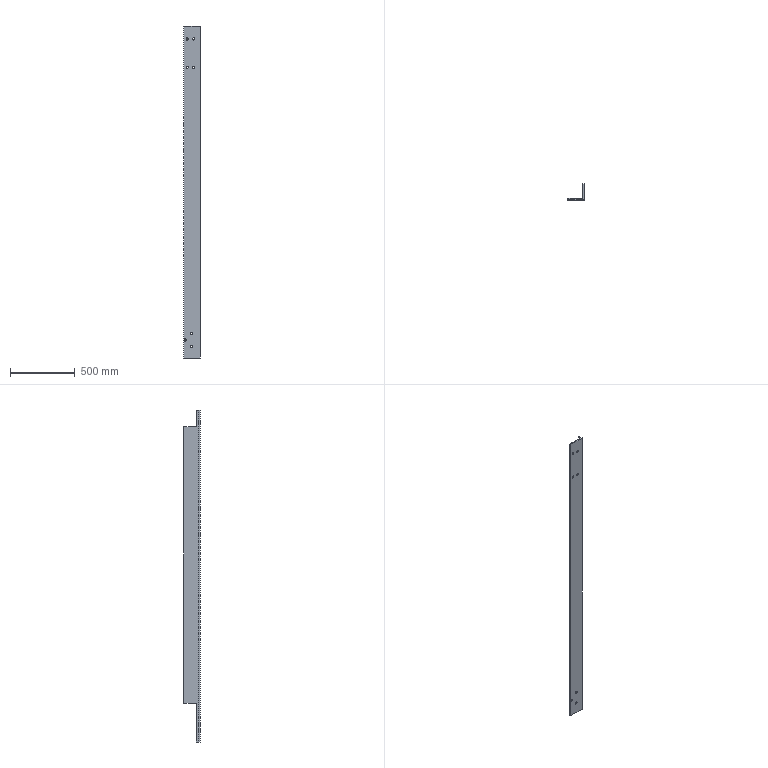Part | SolidWorks | features MirrorStock 1 | 1 solid | 26 faces | box 125 x 125 x 2570 mm | volume 5742663 mm3 | cylinder 14 | plane 12 | commonest cylinder face diameters 17.5 x14
STEP:
#1=CARTESIAN_POINT('',(-100.,0.,956.25));
#2=VERTEX_POINT('',#1);
#3=CARTESIAN_POINT('',(-100.,0.,973.75));
#4=VERTEX_POINT('',#3);
#5=CARTESIAN_POINT('',(-100.,0.,965.));
#6=DIRECTION('',(0.,-1.,0.));
#7=DIRECTION('',(0.,0.,-1.));
#8=AXIS2_PLACEMENT_3D('',#5,#6,#7);
#9=CIRCLE('',#8,8.75);
#10=EDGE_CURVE('',#2,#4,#9,.T.);
#11=ORIENTED_EDGE('',*,*,#10,.T.);
#12=CARTESIAN_POINT('',(-100.,10.,973.75));
#13=VERTEX_POINT('',#12);
#14=CARTESIAN_POINT('',(-100.,10.,973.75));
#15=DIRECTION('',(0.,1.,0.));
#16=VECTOR('',#15,1000.);
#17=LINE('',#14,#16);
#18=EDGE_CURVE('',#4,#13,#17,.T.);
#19=ORIENTED_EDGE('',*,*,#18,.T.);
#20=CARTESIAN_POINT('',(-100.,10.,956.25));
#21=VERTEX_POINT('',#20);
#22=CARTESIAN_POINT('',(-100.,10.,965.));
#23=DIRECTION('',(0.,-1.,0.));
#24=DIRECTION('',(0.,0.,-1.));
#25=AXIS2_PLACEMENT_3D('',#22,#23,#24);
#26=CIRCLE('',#25,8.75);
#27=EDGE_CURVE('',#21,#13,#26,.T.);
#28=ORIENTED_EDGE('',*,*,#27,.F.);
#29=CARTESIAN_POINT('',(-100.,10.,956.25));
#30=DIRECTION('',(0.,1.,0.));
#31=VECTOR('',#30,1000.);
#32=LINE('',#29,#31);
#33=EDGE_CURVE('',#2,#21,#32,.T.);
#34=ORIENTED_EDGE('',*,*,#33,.F.);
#35=EDGE_LOOP('',(#11,#19,#28,#34));
#36=FACE_OUTER_BOUND('',#35,.T.);
#37=CARTESIAN_POINT('',(-100.,10.,965.));
#38=DIRECTION('',(0.,1.,0.));
#39=DIRECTION('',(0.,0.,-1.));
#40=AXIS2_PLACEMENT_3D('',#37,#38,#39);
#41=CYLINDRICAL_SURFACE('',#40,8.75);
#42=ADVANCED_FACE('',(#36),#41,.F.);
#43=CARTESIAN_POINT('',(-50.,0.,956.25));
#44=VERTEX_POINT('',#43);
#45=CARTESIAN_POINT('',(-50.,0.,973.75));
#46=VERTEX_POINT('',#45);
#47=CARTESIAN_POINT('',(-50.,0.,965.));
#48=DIRECTION('',(0.,-1.,0.));
#49=DIRECTION('',(0.,0.,-1.));
#50=AXIS2_PLACEMENT_3D('',#47,#48,#49);
#51=CIRCLE('',#50,8.75);
#52=EDGE_CURVE('',#44,#46,#51,.T.);
#53=ORIENTED_EDGE('',*,*,#52,.T.);
#54=CARTESIAN_POINT('',(-50.,10.,973.75));
#55=VERTEX_POINT('',#54);
#56=CARTESIAN_POINT('',(-50.,10.,973.75));
#57=DIRECTION('',(0.,1.,0.));
#58=VECTOR('',#57,1000.);
#59=LINE('',#56,#58);
#60=EDGE_CURVE('',#46,#55,#59,.T.);
#61=ORIENTED_EDGE('',*,*,#60,.T.);
#62=CARTESIAN_POINT('',(-50.,10.,956.25));
#63=VERTEX_POINT('',#62);
#64=CARTESIAN_POINT('',(-50.,10.,965.));
#65=DIRECTION('',(0.,-1.,0.));
#66=DIRECTION('',(0.,0.,-1.));
#67=AXIS2_PLACEMENT_3D('',#64,#65,#66);
#68=CIRCLE('',#67,8.75);
#69=EDGE_CURVE('',#63,#55,#68,.T.);
#70=ORIENTED_EDGE('',*,*,#69,.F.);
#71=CARTESIAN_POINT('',(-50.,10.,956.25));
#72=DIRECTION('',(0.,1.,0.));
#73=VECTOR('',#72,1000.);
#74=LINE('',#71,#73);
#75=EDGE_CURVE('',#44,#63,#74,.T.);
#76=ORIENTED_EDGE('',*,*,#75,.F.);
#77=EDGE_LOOP('',(#53,#61,#70,#76));
#78=FACE_OUTER_BOUND('',#77,.T.);
#79=CARTESIAN_POINT('',(-50.,10.,965.));
#80=DIRECTION('',(0.,1.,0.));
#81=DIRECTION('',(0.,0.,-1.));
#82=AXIS2_PLACEMENT_3D('',#79,#80,#81);
#83=CYLINDRICAL_SURFACE('',#82,8.75);
#84=ADVANCED_FACE('',(#78),#83,.F.);
#85=CARTESIAN_POINT('',(-50.,0.,1176.25));
#86=VERTEX_POINT('',#85);
#87=CARTESIAN_POINT('',(-50.,0.,1193.75));
#88=VERTEX_POINT('',#87);
#89=CARTESIAN_POINT('',(-50.,0.,1185.));
#90=DIRECTION('',(0.,-1.,0.));
#91=DIRECTION('',(0.,0.,-1.));
#92=AXIS2_PLACEMENT_3D('',#89,#90,#91);
#93=CIRCLE('',#92,8.75);
#94=EDGE_CURVE('',#86,#88,#93,.T.);
#95=ORIENTED_EDGE('',*,*,#94,.T.);
#96=CARTESIAN_POINT('',(-50.,10.,1193.75));
#97=VERTEX_POINT('',#96);
#98=CARTESIAN_POINT('',(-50.,10.,1193.75));
#99=DIRECTION('',(0.,1.,0.));
#100=VECTOR('',#99,1000.);
#101=LINE('',#98,#100);
#102=EDGE_CURVE('',#88,#97,#101,.T.);
#103=ORIENTED_EDGE('',*,*,#102,.T.);
#104=CARTESIAN_POINT('',(-50.,10.,1176.25));
#105=VERTEX_POINT('',#104);
#106=CARTESIAN_POINT('',(-50.,10.,1185.));
#107=DIRECTION('',(0.,-1.,0.));
#108=DIRECTION('',(0.,0.,-1.));
#109=AXIS2_PLACEMENT_3D('',#106,#107,#108);
#110=CIRCLE('',#109,8.75);
#111=EDGE_CURVE('',#105,#97,#110,.T.);
#112=ORIENTED_EDGE('',*,*,#111,.F.);
#113=CARTESIAN_POINT('',(-50.,10.,1176.25));
#114=DIRECTION('',(0.,1.,0.));
#115=VECTOR('',#114,1000.);
#116=LINE('',#113,#115);
#117=EDGE_CURVE('',#86,#105,#116,.T.);
#118=ORIENTED_EDGE('',*,*,#117,.F.);
#119=EDGE_LOOP('',(#95,#103,#112,#118));
#120=FACE_OUTER_BOUND('',#119,.T.);
#121=CARTESIAN_POINT('',(-50.,10.,1185.));
#122=DIRECTION('',(0.,1.,0.));
#123=DIRECTION('',(0.,0.,-1.));
#124=AXIS2_PLACEMENT_3D('',#121,#122,#123);
#125=CYLINDRICAL_SURFACE('',#124,8.75);
#126=ADVANCED_FACE('',(#120),#125,.F.);
#127=CARTESIAN_POINT('',(-100.,0.,1176.25));
#128=VERTEX_POINT('',#127);
#129=CARTESIAN_POINT('',(-100.,0.,1193.75));
#130=VERTEX_POINT('',#129);
#131=CARTESIAN_POINT('',(-100.,0.,1185.));
#132=DIRECTION('',(0.,-1.,0.));
#133=DIRECTION('',(0.,0.,-1.));
#134=AXIS2_PLACEMENT_3D('',#131,#132,#133);
#135=CIRCLE('',#134,8.75);
#136=EDGE_CURVE('',#128,#130,#135,.T.);
#137=ORIENTED_EDGE('',*,*,#136,.T.);
#138=CARTESIAN_POINT('',(-100.,10.,1193.75));
#139=VERTEX_POINT('',#138);
#140=CARTESIAN_POINT('',(-100.,10.,1193.75));
#141=DIRECTION('',(0.,1.,0.));
#142=VECTOR('',#141,1000.);
#143=LINE('',#140,#142);
#144=EDGE_CURVE('',#130,#139,#143,.T.);
#145=ORIENTED_EDGE('',*,*,#144,.T.);
#146=CARTESIAN_POINT('',(-100.,10.,1176.25));
#147=VERTEX_POINT('',#146);
#148=CARTESIAN_POINT('',(-100.,10.,1185.));
#149=DIRECTION('',(0.,-1.,0.));
#150=DIRECTION('',(0.,0.,-1.));
#151=AXIS2_PLACEMENT_3D('',#148,#149,#150);
#152=CIRCLE('',#151,8.75);
#153=EDGE_CURVE('',#147,#139,#152,.T.);
#154=ORIENTED_EDGE('',*,*,#153,.F.);
#155=CARTESIAN_POINT('',(-100.,10.,1176.25));
#156=DIRECTION('',(0.,1.,0.));
#157=VECTOR('',#156,1000.);
#158=LINE('',#155,#157);
#159=EDGE_CURVE('',#128,#147,#158,.T.);
#160=ORIENTED_EDGE('',*,*,#159,.F.);
#161=EDGE_LOOP('',(#137,#145,#154,#160));
#162=FACE_OUTER_BOUND('',#161,.T.);
#163=CARTESIAN_POINT('',(-100.,10.,1185.));
#164=DIRECTION('',(0.,1.,0.));
#165=DIRECTION('',(0.,0.,-1.));
#166=AXIS2_PLACEMENT_3D('',#163,#164,#165);
#167=CYLINDRICAL_SURFACE('',#166,8.75);
#168=ADVANCED_FACE('',(#162),#167,.F.);
#169=CARTESIAN_POINT('',(-115.,0.,-1153.75));
#170=VERTEX_POINT('',#169);
#171=CARTESIAN_POINT('',(-115.,0.,-1136.25));
#172=VERTEX_POINT('',#171);
#173=CARTESIAN_POINT('',(-115.,0.,-1145.));
#174=DIRECTION('',(0.,-1.,0.));
#175=DIRECTION('',(0.,0.,-1.));
#176=AXIS2_PLACEMENT_3D('',#173,#174,#175);
#177=CIRCLE('',#176,8.75);
#178=EDGE_CURVE('',#170,#172,#177,.T.);
#179=ORIENTED_EDGE('',*,*,#178,.T.);
#180=CARTESIAN_POINT('',(-115.,10.,-1136.25));
#181=VERTEX_POINT('',#180);
#182=CARTESIAN_POINT('',(-115.,10.,-1136.25));
#183=DIRECTION('',(0.,1.,0.));
#184=VECTOR('',#183,1000.);
#185=LINE('',#182,#184);
#186=EDGE_CURVE('',#172,#181,#185,.T.);
#187=ORIENTED_EDGE('',*,*,#186,.T.);
#188=CARTESIAN_POINT('',(-115.,10.,-1153.75));
#189=VERTEX_POINT('',#188);
#190=CARTESIAN_POINT('',(-115.,10.,-1145.));
#191=DIRECTION('',(0.,-1.,0.));
#192=DIRECTION('',(0.,0.,-1.));
#193=AXIS2_PLACEMENT_3D('',#190,#191,#192);
#194=CIRCLE('',#193,8.75);
#195=EDGE_CURVE('',#189,#181,#194,.T.);
#196=ORIENTED_EDGE('',*,*,#195,.F.);
#197=CARTESIAN_POINT('',(-115.,10.,-1153.75));
#198=DIRECTION('',(0.,1.,0.));
#199=VECTOR('',#198,1000.);
#200=LINE('',#197,#199);
#201=EDGE_CURVE('',#170,#189,#200,.T.);
#202=ORIENTED_EDGE('',*,*,#201,.F.);
#203=EDGE_LOOP('',(#179,#187,#196,#202));
#204=FACE_OUTER_BOUND('',#203,.T.);
#205=CARTESIAN_POINT('',(-115.,10.,-1145.));
#206=DIRECTION('',(0.,1.,0.));
#207=DIRECTION('',(0.,0.,-1.));
#208=AXIS2_PLACEMENT_3D('',#205,#206,#207);
#209=CYLINDRICAL_SURFACE('',#208,8.75);
#210=ADVANCED_FACE('',(#204),#209,.F.);
#211=CARTESIAN_POINT('',(-65.,0.,-1103.75));
#212=VERTEX_POINT('',#211);
#213=CARTESIAN_POINT('',(-65.,0.,-1086.25));
#214=VERTEX_POINT('',#213);
#215=CARTESIAN_POINT('',(-65.,0.,-1095.));
#216=DIRECTION('',(0.,-1.,0.));
#217=DIRECTION('',(0.,0.,-1.));
#218=AXIS2_PLACEMENT_3D('',#215,#216,#217);
#219=CIRCLE('',#218,8.75);
#220=EDGE_CURVE('',#212,#214,#219,.T.);
#221=ORIENTED_EDGE('',*,*,#220,.T.);
#222=CARTESIAN_POINT('',(-65.,10.,-1086.25));
#223=VERTEX_POINT('',#222);
#224=CARTESIAN_POINT('',(-65.,10.,-1086.25));
#225=DIRECTION('',(0.,1.,0.));
#226=VECTOR('',#225,1000.);
#227=LINE('',#224,#226);
#228=EDGE_CURVE('',#214,#223,#227,.T.);
#229=ORIENTED_EDGE('',*,*,#228,.T.);
#230=CARTESIAN_POINT('',(-65.,10.,-1103.75));
#231=VERTEX_POINT('',#230);
#232=CARTESIAN_POINT('',(-65.,10.,-1095.));
#233=DIRECTION('',(0.,-1.,0.));
#234=DIRECTION('',(0.,0.,-1.));
#235=AXIS2_PLACEMENT_3D('',#232,#233,#234);
#236=CIRCLE('',#235,8.75);
#237=EDGE_CURVE('',#231,#223,#236,.T.);
#238=ORIENTED_EDGE('',*,*,#237,.F.);
#239=CARTESIAN_POINT('',(-65.,10.,-1103.75));
#240=DIRECTION('',(0.,1.,0.));
#241=VECTOR('',#240,1000.);
#242=LINE('',#239,#241);
#243=EDGE_CURVE('',#212,#231,#242,.T.);
#244=ORIENTED_EDGE('',*,*,#243,.F.);
#245=EDGE_LOOP('',(#221,#229,#238,#244));
#246=FACE_OUTER_BOUND('',#245,.T.);
#247=CARTESIAN_POINT('',(-65.,10.,-1095.));
#248=DIRECTION('',(0.,1.,0.));
#249=DIRECTION('',(0.,0.,-1.));
#250=AXIS2_PLACEMENT_3D('',#247,#248,#249);
#251=CYLINDRICAL_SURFACE('',#250,8.75);
#252=ADVANCED_FACE('',(#246),#251,.F.);
#253=CARTESIAN_POINT('',(-65.,0.,-1203.75));
#254=VERTEX_POINT('',#253);
#255=CARTESIAN_POINT('',(-65.,0.,-1186.25));
#256=VERTEX_POINT('',#255);
#257=CARTESIAN_POINT('',(-65.,0.,-1195.));
#258=DIRECTION('',(0.,-1.,0.));
#259=DIRECTION('',(0.,0.,-1.));
#260=AXIS2_PLACEMENT_3D('',#257,#258,#259);
#261=CIRCLE('',#260,8.75);
#262=EDGE_CURVE('',#254,#256,#261,.T.);
#263=ORIENTED_EDGE('',*,*,#262,.T.);
#264=CARTESIAN_POINT('',(-65.,10.,-1186.25));
#265=VERTEX_POINT('',#264);
#266=CARTESIAN_POINT('',(-65.,10.,-1186.25));
#267=DIRECTION('',(0.,1.,0.));
#268=VECTOR('',#267,1000.);
#269=LINE('',#266,#268);
#270=EDGE_CURVE('',#256,#265,#269,.T.);
#271=ORIENTED_EDGE('',*,*,#270,.T.);
#272=CARTESIAN_POINT('',(-65.,10.,-1203.75));
#273=VERTEX_POINT('',#272);
#274=CARTESIAN_POINT('',(-65.,10.,-1195.));
#275=DIRECTION('',(0.,-1.,0.));
#276=DIRECTION('',(0.,0.,-1.));
#277=AXIS2_PLACEMENT_3D('',#274,#275,#276);
#278=CIRCLE('',#277,8.75);
#279=EDGE_CURVE('',#273,#265,#278,.T.);
#280=ORIENTED_EDGE('',*,*,#279,.F.);
#281=CARTESIAN_POINT('',(-65.,10.,-1203.75));
#282=DIRECTION('',(0.,1.,0.));
#283=VECTOR('',#282,1000.);
#284=LINE('',#281,#283);
#285=EDGE_CURVE('',#254,#273,#284,.T.);
#286=ORIENTED_EDGE('',*,*,#285,.F.);
#287=EDGE_LOOP('',(#263,#271,#280,#286));
#288=FACE_OUTER_BOUND('',#287,.T.);
#289=CARTESIAN_POINT('',(-65.,10.,-1195.));
#290=DIRECTION('',(0.,1.,0.));
#291=DIRECTION('',(0.,0.,-1.));
#292=AXIS2_PLACEMENT_3D('',#289,#290,#291);
#293=CYLINDRICAL_SURFACE('',#292,8.75);
#294=ADVANCED_FACE('',(#288),#293,.F.);
#295=CARTESIAN_POINT('',(-125.,10.,1285.));
#296=VERTEX_POINT('',#295);
#297=CARTESIAN_POINT('',(-125.,0.,1285.));
#298=VERTEX_POINT('',#297);
#299=CARTESIAN_POINT('',(-125.,10.,1285.));
#300=DIRECTION('',(0.,-1.,0.));
#301=VECTOR('',#300,1000.);
#302=LINE('',#299,#301);
#303=EDGE_CURVE('',#296,#298,#302,.T.);
#304=ORIENTED_EDGE('',*,*,#303,.F.);
#305=CARTESIAN_POINT('',(-125.,10.,-1285.));
#306=VERTEX_POINT('',#305);
#307=CARTESIAN_POINT('',(-125.,10.,-1285.));
#308=DIRECTION('',(0.,0.,1.));
#309=VECTOR('',#308,1000.);
#310=LINE('',#307,#309);
#311=EDGE_CURVE('',#306,#296,#310,.T.);
#312=ORIENTED_EDGE('',*,*,#311,.F.);
#313=CARTESIAN_POINT('',(-125.,0.,-1285.));
#314=VERTEX_POINT('',#313);
#315=CARTESIAN_POINT('',(-125.,10.,-1285.));
#316=DIRECTION('',(0.,-1.,0.));
#317=VECTOR('',#316,1000.);
#318=LINE('',#315,#317);
#319=EDGE_CURVE('',#306,#314,#318,.T.);
#320=ORIENTED_EDGE('',*,*,#319,.T.);
#321=CARTESIAN_POINT('',(-125.,0.,-1285.));
#322=DIRECTION('',(0.,0.,1.));
#323=VECTOR('',#322,1000.);
#324=LINE('',#321,#323);
#325=EDGE_CURVE('',#314,#298,#324,.T.);
#326=ORIENTED_EDGE('',*,*,#325,.T.);
#327=EDGE_LOOP('',(#304,#312,#320,#326));
#328=FACE_OUTER_BOUND('',#327,.T.);
#329=CARTESIAN_POINT('',(-125.,10.,-1285.));
#330=DIRECTION('',(1.,0.,0.));
#331=DIRECTION('',(0.,0.,1.));
#332=AXIS2_PLACEMENT_3D('',#329,#330,#331);
#333=PLANE('',#332);
#334=ADVANCED_FACE('',(#328),#333,.F.);
#335=ORIENTED_EDGE('',*,*,#10,.F.);
#336=CARTESIAN_POINT('',(-100.,0.,965.));
#337=DIRECTION('',(0.,-1.,0.));
#338=DIRECTION('',(0.,0.,-1.));
#339=AXIS2_PLACEMENT_3D('',#336,#337,#338);
#340=CIRCLE('',#339,8.75);
#341=EDGE_CURVE('',#4,#2,#340,.T.);
#342=ORIENTED_EDGE('',*,*,#341,.F.);
#343=EDGE_LOOP('',(#335,#342));
#344=FACE_BOUND('',#343,.T.);
#345=ORIENTED_EDGE('',*,*,#52,.F.);
#346=CARTESIAN_POINT('',(-50.,0.,965.));
#347=DIRECTION('',(0.,-1.,0.));
#348=DIRECTION('',(0.,0.,-1.));
#349=AXIS2_PLACEMENT_3D('',#346,#347,#348);
#350=CIRCLE('',#349,8.75);
#351=EDGE_CURVE('',#46,#44,#350,.T.);
#352=ORIENTED_EDGE('',*,*,#351,.F.);
#353=EDGE_LOOP('',(#345,#352));
#354=FACE_BOUND('',#353,.T.);
#355=ORIENTED_EDGE('',*,*,#94,.F.);
#356=CARTESIAN_POINT('',(-50.,0.,1185.));
#357=DIRECTION('',(0.,-1.,0.));
#358=DIRECTION('',(0.,0.,-1.));
#359=AXIS2_PLACEMENT_3D('',#356,#357,#358);
#360=CIRCLE('',#359,8.75);
#361=EDGE_CURVE('',#88,#86,#360,.T.);
#362=ORIENTED_EDGE('',*,*,#361,.F.);
#363=EDGE_LOOP('',(#355,#362));
#364=FACE_BOUND('',#363,.T.);
#365=ORIENTED_EDGE('',*,*,#136,.F.);
#366=CARTESIAN_POINT('',(-100.,0.,1185.));
#367=DIRECTION('',(0.,-1.,0.));
#368=DIRECTION('',(0.,0.,-1.));
#369=AXIS2_PLACEMENT_3D('',#366,#367,#368);
#370=CIRCLE('',#369,8.75);
#371=EDGE_CURVE('',#130,#128,#370,.T.);
#372=ORIENTED_EDGE('',*,*,#371,.F.);
#373=EDGE_LOOP('',(#365,#372));
#374=FACE_BOUND('',#373,.T.);
#375=ORIENTED_EDGE('',*,*,#178,.F.);
#376=CARTESIAN_POINT('',(-115.,0.,-1145.));
#377=DIRECTION('',(0.,-1.,0.));
#378=DIRECTION('',(0.,0.,-1.));
#379=AXIS2_PLACEMENT_3D('',#376,#377,#378);
#380=CIRCLE('',#379,8.75);
#381=EDGE_CURVE('',#172,#170,#380,.T.);
#382=ORIENTED_EDGE('',*,*,#381,.F.);
#383=EDGE_LOOP('',(#375,#382));
#384=FACE_BOUND('',#383,.T.);
#385=ORIENTED_EDGE('',*,*,#220,.F.);
#386=CARTESIAN_POINT('',(-65.,0.,-1095.));
#387=DIRECTION('',(0.,-1.,0.));
#388=DIRECTION('',(0.,0.,-1.));
#389=AXIS2_PLACEMENT_3D('',#386,#387,#388);
#390=CIRCLE('',#389,8.75);
#391=EDGE_CURVE('',#214,#212,#390,.T.);
#392=ORIENTED_EDGE('',*,*,#391,.F.);
#393=EDGE_LOOP('',(#385,#392));
#394=FACE_BOUND('',#393,.T.);
#395=ORIENTED_EDGE('',*,*,#262,.F.);
#396=CARTESIAN_POINT('',(-65.,0.,-1195.));
#397=DIRECTION('',(0.,-1.,0.));
#398=DIRECTION('',(0.,0.,-1.));
#399=AXIS2_PLACEMENT_3D('',#396,#397,#398);
#400=CIRCLE('',#399,8.75);
#401=EDGE_CURVE('',#256,#254,#400,.T.);
#402=ORIENTED_EDGE('',*,*,#401,.F.);
#403=EDGE_LOOP('',(#395,#402));
#404=FACE_BOUND('',#403,.T.);
#405=CARTESIAN_POINT('',(0.,0.,1285.));
#406=VERTEX_POINT('',#405);
#407=CARTESIAN_POINT('',(-125.,0.,1285.));
#408=DIRECTION('',(1.,0.,0.));
#409=VECTOR('',#408,1000.);
#410=LINE('',#407,#409);
#411=EDGE_CURVE('',#298,#406,#410,.T.);
#412=ORIENTED_EDGE('',*,*,#411,.F.);
#413=ORIENTED_EDGE('',*,*,#325,.F.);
#414=CARTESIAN_POINT('',(0.,0.,-1285.));
#415=VERTEX_POINT('',#414);
#416=CARTESIAN_POINT('',(-125.,0.,-1285.));
#417=DIRECTION('',(1.,0.,0.));
#418=VECTOR('',#417,1000.);
#419=LINE('',#416,#418);
#420=EDGE_CURVE('',#314,#415,#419,.T.);
#421=ORIENTED_EDGE('',*,*,#420,.T.);
#422=CARTESIAN_POINT('',(0.,0.,-1285.));
#423=DIRECTION('',(0.,0.,1.));
#424=VECTOR('',#423,1000.);
#425=LINE('',#422,#424);
#426=EDGE_CURVE('',#415,#406,#425,.T.);
#427=ORIENTED_EDGE('',*,*,#426,.T.);
#428=EDGE_LOOP('',(#412,#413,#421,#427));
#429=FACE_OUTER_BOUND('',#428,.T.);
#430=CARTESIAN_POINT('',(-125.,0.,-1285.));
#431=DIRECTION('',(0.,1.,0.));
#432=DIRECTION('',(0.,0.,-1.));
#433=AXIS2_PLACEMENT_3D('',#430,#431,#432);
#434=PLANE('',#433);
#435=ADVANCED_FACE('',(#344,#354,#364,#374,#384,#394,#404,#429),#434,.F.);
#436=CARTESIAN_POINT('',(0.,125.,-985.));
#437=VERTEX_POINT('',#436);
#438=CARTESIAN_POINT('',(0.,30.,-985.));
#439=VERTEX_POINT('',#438);
#440=CARTESIAN_POINT('',(0.,125.,-985.));
#441=DIRECTION('',(0.,-1.,0.));
#442=VECTOR('',#441,1000.);
#443=LINE('',#440,#442);
#444=EDGE_CURVE('',#437,#439,#443,.T.);
#445=ORIENTED_EDGE('',*,*,#444,.F.);
#446=CARTESIAN_POINT('',(0.,125.,1155.));
#447=VERTEX_POINT('',#446);
#448=CARTESIAN_POINT('',(0.,125.,-1285.));
#449=DIRECTION('',(0.,0.,1.));
#450=VECTOR('',#449,1000.);
#451=LINE('',#448,#450);
#452=EDGE_CURVE('',#437,#447,#451,.T.);
#453=ORIENTED_EDGE('',*,*,#452,.T.);
#454=CARTESIAN_POINT('',(0.,30.,1155.));
#455=VERTEX_POINT('',#454);
#456=CARTESIAN_POINT('',(0.,125.,1155.));
#457=DIRECTION('',(0.,1.,0.));
#458=VECTOR('',#457,1000.);
#459=LINE('',#456,#458);
#460=EDGE_CURVE('',#455,#447,#459,.T.);
#461=ORIENTED_EDGE('',*,*,#460,.F.);
#462=CARTESIAN_POINT('',(0.,30.,1285.));
#463=VERTEX_POINT('',#462);
#464=CARTESIAN_POINT('',(0.,30.,1285.));
#465=DIRECTION('',(0.,0.,-1.));
#466=VECTOR('',#465,1000.);
#467=LINE('',#464,#466);
#468=EDGE_CURVE('',#463,#455,#467,.T.);
#469=ORIENTED_EDGE('',*,*,#468,.F.);
#470=CARTESIAN_POINT('',(0.,0.,1285.));
#471=DIRECTION('',(0.,1.,0.));
#472=VECTOR('',#471,1000.);
#473=LINE('',#470,#472);
#474=EDGE_CURVE('',#406,#463,#473,.T.);
#475=ORIENTED_EDGE('',*,*,#474,.F.);
#476=ORIENTED_EDGE('',*,*,#426,.F.);
#477=CARTESIAN_POINT('',(0.,30.,-1285.));
#478=VERTEX_POINT('',#477);
#479=CARTESIAN_POINT('',(0.,0.,-1285.));
#480=DIRECTION('',(0.,1.,0.));
#481=VECTOR('',#480,1000.);
#482=LINE('',#479,#481);
#483=EDGE_CURVE('',#415,#478,#482,.T.);
#484=ORIENTED_EDGE('',*,*,#483,.T.);
#485=CARTESIAN_POINT('',(0.,30.,-1285.));
#486=DIRECTION('',(0.,0.,-1.));
#487=VECTOR('',#486,1000.);
#488=LINE('',#485,#487);
#489=EDGE_CURVE('',#439,#478,#488,.T.);
#490=ORIENTED_EDGE('',*,*,#489,.F.);
#491=EDGE_LOOP('',(#445,#453,#461,#469,#475,#476,#484,#490));
#492=FACE_OUTER_BOUND('',#491,.T.);
#493=CARTESIAN_POINT('',(0.,0.,-1285.));
#494=DIRECTION('',(-1.,0.,0.));
#495=DIRECTION('',(0.,0.,-1.));
#496=AXIS2_PLACEMENT_3D('',#493,#494,#495);
#497=PLANE('',#496);
#498=ADVANCED_FACE('',(#492),#497,.F.);
#499=CARTESIAN_POINT('',(-10.,125.,-985.));
#500=VERTEX_POINT('',#499);
#501=CARTESIAN_POINT('',(-10.,125.,1155.));
#502=VERTEX_POINT('',#501);
#503=CARTESIAN_POINT('',(-10.,125.,-1285.));
#504=DIRECTION('',(0.,0.,1.));
#505=VECTOR('',#504,1000.);
#506=LINE('',#503,#505);
#507=EDGE_CURVE('',#500,#502,#506,.T.);
#508=ORIENTED_EDGE('',*,*,#507,.T.);
#509=CARTESIAN_POINT('',(0.,125.,1155.));
#510=DIRECTION('',(-1.,0.,0.));
#511=VECTOR('',#510,1000.);
#512=LINE('',#509,#511);
#513=EDGE_CURVE('',#447,#502,#512,.T.);
#514=ORIENTED_EDGE('',*,*,#513,.F.);
#515=ORIENTED_EDGE('',*,*,#452,.F.);
#516=CARTESIAN_POINT('',(0.,125.,-985.));
#517=DIRECTION('',(-1.,0.,0.));
#518=VECTOR('',#517,1000.);
#519=LINE('',#516,#518);
#520=EDGE_CURVE('',#437,#500,#519,.T.);
#521=ORIENTED_EDGE('',*,*,#520,.T.);
#522=EDGE_LOOP('',(#508,#514,#515,#521));
#523=FACE_OUTER_BOUND('',#522,.T.);
#524=CARTESIAN_POINT('',(-10.,125.,-1285.));
#525=DIRECTION('',(0.,-1.,0.));
#526=DIRECTION('',(0.,0.,1.));
#527=AXIS2_PLACEMENT_3D('',#524,#525,#526);
#528=PLANE('',#527);
#529=ADVANCED_FACE('',(#523),#528,.F.);
#530=CARTESIAN_POINT('',(-10.,30.,-1285.));
#531=VERTEX_POINT('',#530);
#532=CARTESIAN_POINT('',(-10.,10.,-1285.));
#533=VERTEX_POINT('',#532);
#534=CARTESIAN_POINT('',(-10.,10.,-1285.));
#535=DIRECTION('',(0.,-1.,0.));
#536=VECTOR('',#535,1000.);
#537=LINE('',#534,#536);
#538=EDGE_CURVE('',#531,#533,#537,.T.);
#539=ORIENTED_EDGE('',*,*,#538,.T.);
#540=CARTESIAN_POINT('',(-10.,10.,1285.));
#541=VERTEX_POINT('',#540);
#542=CARTESIAN_POINT('',(-10.,10.,-1285.));
#543=DIRECTION('',(0.,0.,1.));
#544=VECTOR('',#543,1000.);
#545=LINE('',#542,#544);
#546=EDGE_CURVE('',#533,#541,#545,.T.);
#547=ORIENTED_EDGE('',*,*,#546,.T.);
#548=CARTESIAN_POINT('',(-10.,30.,1285.));
#549=VERTEX_POINT('',#548);
#550=CARTESIAN_POINT('',(-10.,10.,1285.));
#551=DIRECTION('',(0.,-1.,0.));
#552=VECTOR('',#551,1000.);
#553=LINE('',#550,#552);
#554=EDGE_CURVE('',#549,#541,#553,.T.);
#555=ORIENTED_EDGE('',*,*,#554,.F.);
#556=CARTESIAN_POINT('',(-10.,30.,1155.));
#557=VERTEX_POINT('',#556);
#558=CARTESIAN_POINT('',(-10.,30.,1285.));
#559=DIRECTION('',(0.,0.,-1.));
#560=VECTOR('',#559,1000.);
#561=LINE('',#558,#560);
#562=EDGE_CURVE('',#549,#557,#561,.T.);
#563=ORIENTED_EDGE('',*,*,#562,.T.);
#564=CARTESIAN_POINT('',(-10.,125.,1155.));
#565=DIRECTION('',(0.,1.,0.));
#566=VECTOR('',#565,1000.);
#567=LINE('',#564,#566);
#568=EDGE_CURVE('',#557,#502,#567,.T.);
#569=ORIENTED_EDGE('',*,*,#568,.T.);
#570=ORIENTED_EDGE('',*,*,#507,.F.);
#571=CARTESIAN_POINT('',(-10.,30.,-985.));
#572=VERTEX_POINT('',#571);
#573=CARTESIAN_POINT('',(-10.,125.,-985.));
#574=DIRECTION('',(0.,-1.,0.));
#575=VECTOR('',#574,1000.);
#576=LINE('',#573,#575);
#577=EDGE_CURVE('',#500,#572,#576,.T.);
#578=ORIENTED_EDGE('',*,*,#577,.T.);
#579=CARTESIAN_POINT('',(-10.,30.,-1285.));
#580=DIRECTION('',(0.,0.,-1.));
#581=VECTOR('',#580,1000.);
#582=LINE('',#579,#581);
#583=EDGE_CURVE('',#572,#531,#582,.T.);
#584=ORIENTED_EDGE('',*,*,#583,.T.);
#585=EDGE_LOOP('',(#539,#547,#555,#563,#569,#570,#578,#584));
#586=FACE_OUTER_BOUND('',#585,.T.);
#587=CARTESIAN_POINT('',(-10.,10.,-1285.));
#588=DIRECTION('',(1.,0.,0.));
#589=DIRECTION('',(0.,0.,1.));
#590=AXIS2_PLACEMENT_3D('',#587,#588,#589);
#591=PLANE('',#590);
#592=ADVANCED_FACE('',(#586),#591,.F.);
#593=ORIENTED_EDGE('',*,*,#27,.T.);
#594=CARTESIAN_POINT('',(-100.,10.,965.));
#595=DIRECTION('',(0.,-1.,0.));
#596=DIRECTION('',(0.,0.,-1.));
#597=AXIS2_PLACEMENT_3D('',#594,#595,#596);
#598=CIRCLE('',#597,8.75);
#599=EDGE_CURVE('',#13,#21,#598,.T.);
#600=ORIENTED_EDGE('',*,*,#599,.T.);
#601=EDGE_LOOP('',(#593,#600));
#602=FACE_BOUND('',#601,.T.);
#603=ORIENTED_EDGE('',*,*,#69,.T.);
#604=CARTESIAN_POINT('',(-50.,10.,965.));
#605=DIRECTION('',(0.,-1.,0.));
#606=DIRECTION('',(0.,0.,-1.));
#607=AXIS2_PLACEMENT_3D('',#604,#605,#606);
#608=CIRCLE('',#607,8.75);
#609=EDGE_CURVE('',#55,#63,#608,.T.);
#610=ORIENTED_EDGE('',*,*,#609,.T.);
#611=EDGE_LOOP('',(#603,#610));
#612=FACE_BOUND('',#611,.T.);
#613=ORIENTED_EDGE('',*,*,#111,.T.);
#614=CARTESIAN_POINT('',(-50.,10.,1185.));
#615=DIRECTION('',(0.,-1.,0.));
#616=DIRECTION('',(0.,0.,-1.));
#617=AXIS2_PLACEMENT_3D('',#614,#615,#616);
#618=CIRCLE('',#617,8.75);
#619=EDGE_CURVE('',#97,#105,#618,.T.);
#620=ORIENTED_EDGE('',*,*,#619,.T.);
#621=EDGE_LOOP('',(#613,#620));
#622=FACE_BOUND('',#621,.T.);
#623=ORIENTED_EDGE('',*,*,#153,.T.);
#624=CARTESIAN_POINT('',(-100.,10.,1185.));
#625=DIRECTION('',(0.,-1.,0.));
#626=DIRECTION('',(0.,0.,-1.));
#627=AXIS2_PLACEMENT_3D('',#624,#625,#626);
#628=CIRCLE('',#627,8.75);
#629=EDGE_CURVE('',#139,#147,#628,.T.);
#630=ORIENTED_EDGE('',*,*,#629,.T.);
#631=EDGE_LOOP('',(#623,#630));
#632=FACE_BOUND('',#631,.T.);
#633=ORIENTED_EDGE('',*,*,#195,.T.);
#634=CARTESIAN_POINT('',(-115.,10.,-1145.));
#635=DIRECTION('',(0.,-1.,0.));
#636=DIRECTION('',(0.,0.,-1.));
#637=AXIS2_PLACEMENT_3D('',#634,#635,#636);
#638=CIRCLE('',#637,8.75);
#639=EDGE_CURVE('',#181,#189,#638,.T.);
#640=ORIENTED_EDGE('',*,*,#639,.T.);
#641=EDGE_LOOP('',(#633,#640));
#642=FACE_BOUND('',#641,.T.);
#643=ORIENTED_EDGE('',*,*,#237,.T.);
#644=CARTESIAN_POINT('',(-65.,10.,-1095.));
#645=DIRECTION('',(0.,-1.,0.));
#646=DIRECTION('',(0.,0.,-1.));
#647=AXIS2_PLACEMENT_3D('',#644,#645,#646);
#648=CIRCLE('',#647,8.75);
#649=EDGE_CURVE('',#223,#231,#648,.T.);
#650=ORIENTED_EDGE('',*,*,#649,.T.);
#651=EDGE_LOOP('',(#643,#650));
#652=FACE_BOUND('',#651,.T.);
#653=ORIENTED_EDGE('',*,*,#279,.T.);
#654=CARTESIAN_POINT('',(-65.,10.,-1195.));
#655=DIRECTION('',(0.,-1.,0.));
#656=DIRECTION('',(0.,0.,-1.));
#657=AXIS2_PLACEMENT_3D('',#654,#655,#656);
#658=CIRCLE('',#657,8.75);
#659=EDGE_CURVE('',#265,#273,#658,.T.);
#660=ORIENTED_EDGE('',*,*,#659,.T.);
#661=EDGE_LOOP('',(#653,#660));
#662=FACE_BOUND('',#661,.T.);
#663=CARTESIAN_POINT('',(-125.,10.,1285.));
#664=DIRECTION('',(-1.,0.,0.));
#665=VECTOR('',#664,1000.);
#666=LINE('',#663,#665);
#667=EDGE_CURVE('',#541,#296,#666,.T.);
#668=ORIENTED_EDGE('',*,*,#667,.F.);
#669=ORIENTED_EDGE('',*,*,#546,.F.);
#670=CARTESIAN_POINT('',(-125.,10.,-1285.));
#671=DIRECTION('',(-1.,0.,0.));
#672=VECTOR('',#671,1000.);
#673=LINE('',#670,#672);
#674=EDGE_CURVE('',#533,#306,#673,.T.);
#675=ORIENTED_EDGE('',*,*,#674,.T.);
#676=ORIENTED_EDGE('',*,*,#311,.T.);
#677=EDGE_LOOP('',(#668,#669,#675,#676));
#678=FACE_OUTER_BOUND('',#677,.T.);
#679=CARTESIAN_POINT('',(-125.,10.,-1285.));
#680=DIRECTION('',(0.,-1.,0.));
#681=DIRECTION('',(0.,0.,1.));
#682=AXIS2_PLACEMENT_3D('',#679,#680,#681);
#683=PLANE('',#682);
#684=ADVANCED_FACE('',(#602,#612,#622,#632,#642,#652,#662,#678),#683,.F.);
#685=CARTESIAN_POINT('',(0.,30.,-1285.));
#686=DIRECTION('',(-1.,0.,0.));
#687=VECTOR('',#686,1000.);
#688=LINE('',#685,#687);
#689=EDGE_CURVE('',#478,#531,#688,.T.);
#690=ORIENTED_EDGE('',*,*,#689,.F.);
#691=ORIENTED_EDGE('',*,*,#483,.F.);
#692=ORIENTED_EDGE('',*,*,#420,.F.);
#693=ORIENTED_EDGE('',*,*,#319,.F.);
#694=ORIENTED_EDGE('',*,*,#674,.F.);
#695=ORIENTED_EDGE('',*,*,#538,.F.);
#696=EDGE_LOOP('',(#690,#691,#692,#693,#694,#695));
#697=FACE_OUTER_BOUND('',#696,.T.);
#698=CARTESIAN_POINT('',(0.,0.,-1285.));
#699=DIRECTION('',(0.,0.,-1.));
#700=DIRECTION('',(1.,0.,0.));
#701=AXIS2_PLACEMENT_3D('',#698,#699,#700);
#702=PLANE('',#701);
#703=ADVANCED_FACE('',(#697),#702,.T.);
#704=ORIENTED_EDGE('',*,*,#554,.T.);
#705=ORIENTED_EDGE('',*,*,#667,.T.);
#706=ORIENTED_EDGE('',*,*,#303,.T.);
#707=ORIENTED_EDGE('',*,*,#411,.T.);
#708=ORIENTED_EDGE('',*,*,#474,.T.);
#709=CARTESIAN_POINT('',(0.,30.,1285.));
#710=DIRECTION('',(-1.,0.,0.));
#711=VECTOR('',#710,1000.);
#712=LINE('',#709,#711);
#713=EDGE_CURVE('',#463,#549,#712,.T.);
#714=ORIENTED_EDGE('',*,*,#713,.T.);
#715=EDGE_LOOP('',(#704,#705,#706,#707,#708,#714));
#716=FACE_OUTER_BOUND('',#715,.T.);
#717=CARTESIAN_POINT('',(0.,0.,1285.));
#718=DIRECTION('',(0.,0.,-1.));
#719=DIRECTION('',(1.,0.,0.));
#720=AXIS2_PLACEMENT_3D('',#717,#718,#719);
#721=PLANE('',#720);
#722=ADVANCED_FACE('',(#716),#721,.F.);
#723=ORIENTED_EDGE('',*,*,#270,.F.);
#724=ORIENTED_EDGE('',*,*,#401,.T.);
#725=ORIENTED_EDGE('',*,*,#285,.T.);
#726=ORIENTED_EDGE('',*,*,#659,.F.);
#727=EDGE_LOOP('',(#723,#724,#725,#726));
#728=FACE_OUTER_BOUND('',#727,.T.);
#729=CARTESIAN_POINT('',(-65.,10.,-1195.));
#730=DIRECTION('',(0.,1.,0.));
#731=DIRECTION('',(0.,0.,-1.));
#732=AXIS2_PLACEMENT_3D('',#729,#730,#731);
#733=CYLINDRICAL_SURFACE('',#732,8.75);
#734=ADVANCED_FACE('',(#728),#733,.F.);
#735=ORIENTED_EDGE('',*,*,#228,.F.);
#736=ORIENTED_EDGE('',*,*,#391,.T.);
#737=ORIENTED_EDGE('',*,*,#243,.T.);
#738=ORIENTED_EDGE('',*,*,#649,.F.);
#739=EDGE_LOOP('',(#735,#736,#737,#738));
#740=FACE_OUTER_BOUND('',#739,.T.);
#741=CARTESIAN_POINT('',(-65.,10.,-1095.));
#742=DIRECTION('',(0.,1.,0.));
#743=DIRECTION('',(0.,0.,-1.));
#744=AXIS2_PLACEMENT_3D('',#741,#742,#743);
#745=CYLINDRICAL_SURFACE('',#744,8.75);
#746=ADVANCED_FACE('',(#740),#745,.F.);
#747=ORIENTED_EDGE('',*,*,#186,.F.);
#748=ORIENTED_EDGE('',*,*,#381,.T.);
#749=ORIENTED_EDGE('',*,*,#201,.T.);
#750=ORIENTED_EDGE('',*,*,#639,.F.);
#751=EDGE_LOOP('',(#747,#748,#749,#750));
#752=FACE_OUTER_BOUND('',#751,.T.);
#753=CARTESIAN_POINT('',(-115.,10.,-1145.));
#754=DIRECTION('',(0.,1.,0.));
#755=DIRECTION('',(0.,0.,-1.));
#756=AXIS2_PLACEMENT_3D('',#753,#754,#755);
#757=CYLINDRICAL_SURFACE('',#756,8.75);
#758=ADVANCED_FACE('',(#752),#757,.F.);
#759=ORIENTED_EDGE('',*,*,#144,.F.);
#760=ORIENTED_EDGE('',*,*,#371,.T.);
#761=ORIENTED_EDGE('',*,*,#159,.T.);
#762=ORIENTED_EDGE('',*,*,#629,.F.);
#763=EDGE_LOOP('',(#759,#760,#761,#762));
#764=FACE_OUTER_BOUND('',#763,.T.);
#765=CARTESIAN_POINT('',(-100.,10.,1185.));
#766=DIRECTION('',(0.,1.,0.));
#767=DIRECTION('',(0.,0.,-1.));
#768=AXIS2_PLACEMENT_3D('',#765,#766,#767);
#769=CYLINDRICAL_SURFACE('',#768,8.75);
#770=ADVANCED_FACE('',(#764),#769,.F.);
#771=ORIENTED_EDGE('',*,*,#102,.F.);
#772=ORIENTED_EDGE('',*,*,#361,.T.);
#773=ORIENTED_EDGE('',*,*,#117,.T.);
#774=ORIENTED_EDGE('',*,*,#619,.F.);
#775=EDGE_LOOP('',(#771,#772,#773,#774));
#776=FACE_OUTER_BOUND('',#775,.T.);
#777=CARTESIAN_POINT('',(-50.,10.,1185.));
#778=DIRECTION('',(0.,1.,0.));
#779=DIRECTION('',(0.,0.,-1.));
#780=AXIS2_PLACEMENT_3D('',#777,#778,#779);
#781=CYLINDRICAL_SURFACE('',#780,8.75);
#782=ADVANCED_FACE('',(#776),#781,.F.);
#783=ORIENTED_EDGE('',*,*,#60,.F.);
#784=ORIENTED_EDGE('',*,*,#351,.T.);
#785=ORIENTED_EDGE('',*,*,#75,.T.);
#786=ORIENTED_EDGE('',*,*,#609,.F.);
#787=EDGE_LOOP('',(#783,#784,#785,#786));
#788=FACE_OUTER_BOUND('',#787,.T.);
#789=CARTESIAN_POINT('',(-50.,10.,965.));
#790=DIRECTION('',(0.,1.,0.));
#791=DIRECTION('',(0.,0.,-1.));
#792=AXIS2_PLACEMENT_3D('',#789,#790,#791);
#793=CYLINDRICAL_SURFACE('',#792,8.75);
#794=ADVANCED_FACE('',(#788),#793,.F.);
#795=ORIENTED_EDGE('',*,*,#18,.F.);
#796=ORIENTED_EDGE('',*,*,#341,.T.);
#797=ORIENTED_EDGE('',*,*,#33,.T.);
#798=ORIENTED_EDGE('',*,*,#599,.F.);
#799=EDGE_LOOP('',(#795,#796,#797,#798));
#800=FACE_OUTER_BOUND('',#799,.T.);
#801=CARTESIAN_POINT('',(-100.,10.,965.));
#802=DIRECTION('',(0.,1.,0.));
#803=DIRECTION('',(0.,0.,-1.));
#804=AXIS2_PLACEMENT_3D('',#801,#802,#803);
#805=CYLINDRICAL_SURFACE('',#804,8.75);
#806=ADVANCED_FACE('',(#800),#805,.F.);
#807=ORIENTED_EDGE('',*,*,#568,.F.);
#808=CARTESIAN_POINT('',(0.,30.,1155.));
#809=DIRECTION('',(-1.,0.,0.));
#810=VECTOR('',#809,1000.);
#811=LINE('',#808,#810);
#812=EDGE_CURVE('',#455,#557,#811,.T.);
#813=ORIENTED_EDGE('',*,*,#812,.F.);
#814=ORIENTED_EDGE('',*,*,#460,.T.);
#815=ORIENTED_EDGE('',*,*,#513,.T.);
#816=EDGE_LOOP('',(#807,#813,#814,#815));
#817=FACE_OUTER_BOUND('',#816,.T.);
#818=CARTESIAN_POINT('',(0.,125.,1155.));
#819=DIRECTION('',(0.,0.,-1.));
#820=DIRECTION('',(1.,0.,0.));
#821=AXIS2_PLACEMENT_3D('',#818,#819,#820);
#822=PLANE('',#821);
#823=ADVANCED_FACE('',(#817),#822,.F.);
#824=ORIENTED_EDGE('',*,*,#562,.F.);
#825=ORIENTED_EDGE('',*,*,#713,.F.);
#826=ORIENTED_EDGE('',*,*,#468,.T.);
#827=ORIENTED_EDGE('',*,*,#812,.T.);
#828=EDGE_LOOP('',(#824,#825,#826,#827));
#829=FACE_OUTER_BOUND('',#828,.T.);
#830=CARTESIAN_POINT('',(0.,30.,1285.));
#831=DIRECTION('',(0.,-1.,0.));
#832=DIRECTION('',(0.,0.,1.));
#833=AXIS2_PLACEMENT_3D('',#830,#831,#832);
#834=PLANE('',#833);
#835=ADVANCED_FACE('',(#829),#834,.F.);
#836=ORIENTED_EDGE('',*,*,#583,.F.);
#837=CARTESIAN_POINT('',(0.,30.,-985.));
#838=DIRECTION('',(-1.,0.,0.));
#839=VECTOR('',#838,1000.);
#840=LINE('',#837,#839);
#841=EDGE_CURVE('',#439,#572,#840,.T.);
#842=ORIENTED_EDGE('',*,*,#841,.F.);
#843=ORIENTED_EDGE('',*,*,#489,.T.);
#844=ORIENTED_EDGE('',*,*,#689,.T.);
#845=EDGE_LOOP('',(#836,#842,#843,#844));
#846=FACE_OUTER_BOUND('',#845,.T.);
#847=CARTESIAN_POINT('',(0.,30.,-1285.));
#848=DIRECTION('',(0.,-1.,0.));
#849=DIRECTION('',(0.,0.,1.));
#850=AXIS2_PLACEMENT_3D('',#847,#848,#849);
#851=PLANE('',#850);
#852=ADVANCED_FACE('',(#846),#851,.F.);
#853=ORIENTED_EDGE('',*,*,#577,.F.);
#854=ORIENTED_EDGE('',*,*,#520,.F.);
#855=ORIENTED_EDGE('',*,*,#444,.T.);
#856=ORIENTED_EDGE('',*,*,#841,.T.);
#857=EDGE_LOOP('',(#853,#854,#855,#856));
#858=FACE_OUTER_BOUND('',#857,.T.);
#859=CARTESIAN_POINT('',(0.,125.,-985.));
#860=DIRECTION('',(0.,0.,1.));
#861=DIRECTION('',(-1.,0.,0.));
#862=AXIS2_PLACEMENT_3D('',#859,#860,#861);
#863=PLANE('',#862);
#864=ADVANCED_FACE('',(#858),#863,.F.);
#865=CLOSED_SHELL('',(#42,#84,#126,#168,#210,#252,#294,#334,#435,#498,#529,#592,#684,#703,#722,#734,#746,#758,#770,#782,#794,#806,#823,#835,#852,#864));
#866=MANIFOLD_SOLID_BREP('',#865);
#867=CARTESIAN_POINT('',(0.,0.,0.));
#868=DIRECTION('',(0.,0.,1.));
#869=DIRECTION('',(1.,0.,0.));
#870=AXIS2_PLACEMENT_3D('',#867,#868,#869);
#871=(LENGTH_UNIT()NAMED_UNIT(*)SI_UNIT(.MILLI.,.METRE.));
#872=UNCERTAINTY_MEASURE_WITH_UNIT(LENGTH_MEASURE(0.00001),#871,'','');
#873=(NAMED_UNIT(*)PLANE_ANGLE_UNIT()SI_UNIT($,.RADIAN.));
#874=(NAMED_UNIT(*)SI_UNIT($,.STERADIAN.)SOLID_ANGLE_UNIT());
#875=(GEOMETRIC_REPRESENTATION_CONTEXT(3)GLOBAL_UNCERTAINTY_ASSIGNED_CONTEXT((#872))GLOBAL_UNIT_ASSIGNED_CONTEXT((#871,#873,#874))REPRESENTATION_CONTEXT('',''));
#876=ADVANCED_BREP_SHAPE_REPRESENTATION('',(#866,#870),#875);